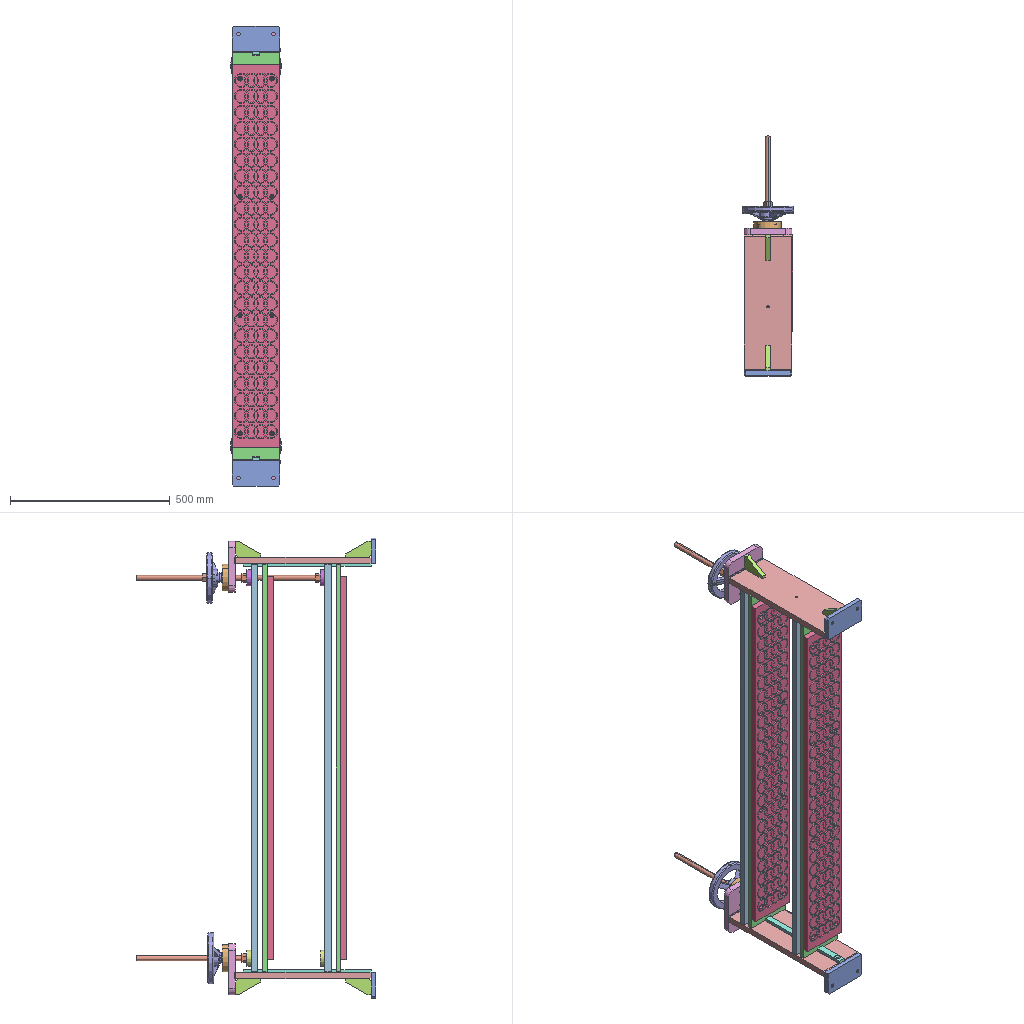Assembly | SolidWorks | 18 different items | 44 placed | box 160 x 749 x 1440 mm
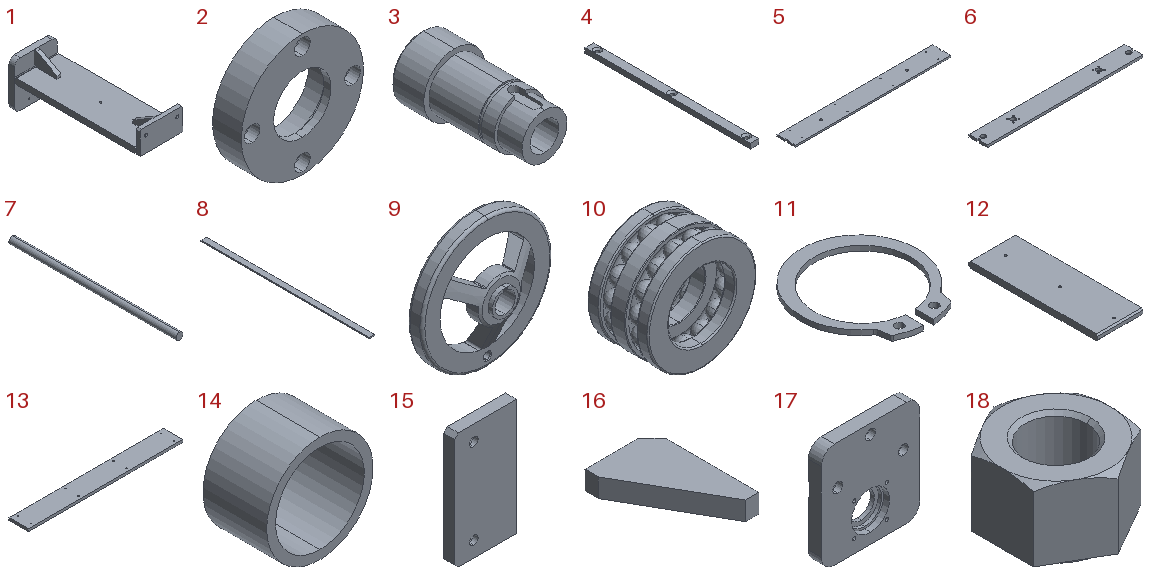Parts list (item | name | quantity | parent item | size | volume | features):
1 | (subassembly) | x2 | - | 150 x 460 x 170 mm | 1894202 mm3 | -
2 | - | x2 | - | 85 x 22 x 85 mm | 70234 mm3 | features ICE 4, Extrusion 1, HoleWzd 1
3 | - | x2 | - | 30 x 60 x 30 mm | 20081 mm3 | features ICE 3, Chamfer 1, HoleWzd 1, RevCut 1, Revolution 1
4 | - | x2 | in 1 | 20 x 400 x 12 mm | 92676 mm3 | features Extrusion 1, HoleWzd 1
5 | - | x2 | - | 1272 x 150 x 14 mm | 2656478 mm3 | features 3DProfileFeature 1, Extrusion 1, HoleWzd 1, ICE 1
6 | - | x2 | - | 1276 x 150 x 34 mm | 3757893 mm3 | features ICE 3, Cut 1, Extrusion 1
7 | - | x3 | - | 16 x 380 x 16 mm | 76404 mm3 | features Extrusion 1
8 | - | x2 | - | 10 x 300 x 2 mm | 6000 mm3 | features Extrusion 1
9 | - | x2 | - | 160 x 40 x 160 mm | 222311 mm3 | features ICE 4, MBimport 1
10 | - | x2 | - | 52 x 29 x 52 mm | 31888 mm3 | features Revolution 2, CirPattern 1
11 | - | x2 | - | 28.2 x 30.881 x 1.2 mm | 272.247 mm3 | features Extrusion 1
12 | - | x2 | in 1 | 150 x 426 x 20 mm | 1243356 mm3 | features Chamfer 2, HoleWzd 2, Extrusion 1, ICE 1
13 | - | x2 | - | 1200 x 150 x 20 mm | 3476597 mm3 | features LPattern 2, Extrusion 1, HoleWzd 1, ICE 1
14 | - | x2 | - | 30 x 18 x 30 mm | 3888 mm3 | features Extrusion 1
15 | - | x2 | in 1 | 80 x 14 x 150 mm | 162438 mm3 | features Chamfer 1, Extrusion 1, HoleWzd 1
16 | - | x4 | in 1 | 50 x 80 x 14 mm | 35700 mm3 | features Chamfer 1, Extrusion 1
17 | - | x2 | in 1 | 150 x 20 x 160 mm | 417009 mm3 | features ICE 4, HoleWzd 2, Extrusion 1, Fillet 1
18 | - | x7 | - | 24 x 27.713 x 16.4 mm | 5589 mm3 | features Cut 2, Chamfer 1, Extrusion 1
Mates (type | each side: item.copy, entity, surface, feature):
In the top assembly
Coincident | 12.1 face plane Boss-Extrude1 | 12.2 face plane Boss-Extrude1
Coincident | 15.1 face plane Boss-Extrude1 | 15.2 face plane Boss-Extrude1
Coincident | 17.1 face plane Boss-Extrude1 | 2.1 face plane Boss-Extrude1
Concentric | 17.1 face cylinder M6 Tapped Hole1 | 2.1 face cylinder M6 Clearance Hole1
Coincident | 17.2 face plane Boss-Extrude1 | 2.2 face plane Boss-Extrude1
Concentric | 17.2 face cylinder M6 Tapped Hole1 | 2.2 face cylinder M6 Clearance Hole1
DistanceDim | 6.1 face plane Boss-Extrude1 | 12.2 face plane Boss-Extrude1
DistanceDim | 6.1 face plane Boss-Extrude1 | 12.1 face plane Boss-Extrude1
Coincident | 12.2 face plane Boss-Extrude1 | 6.1 face plane Boss-Extrude1
DistanceDim | 6.1 face plane Boss-Extrude1 | 5.1 face plane Boss-Extrude1
Coincident | 6.1 face plane Boss-Extrude1 | 5.1 face plane Boss-Extrude1
Coincident | 5.1 face plane Boss-Extrude1 | 13.1 face plane Boss-Extrude1
Concentric | 5.1 face cylinder M8 Tapped Hole1 | 13.1 face cylinder Hole size (by socket head cap screw type)1 | 2 times
LimitDistanceDim | 13.1 face plane Boss-Extrude1 | 15.1 face plane Boss-Extrude1
Concentric | 6.1 face cylinder Cut-Extrude3 | 7.1 face cylinder Boss-Extrude1
DistanceDim | 7.1 face plane Boss-Extrude1 | 6.1 face plane Boss-Extrude1
Concentric | 6.1 face cylinder Cut-Extrude3 | 7.2 face cylinder Boss-Extrude1
Coincident | 7.1 face plane Boss-Extrude1 | 7.2 face plane Boss-Extrude1
Coincident | 17.1 face plane Cut-Extrude1 | 10.1 face plane Revolve1
Concentric | 17.1 face cylinder Cut-Extrude1 | 10.1 face cylinder Revolve1
Concentric | 17.2 face cylinder Cut-Extrude2 | 2.2 face cylinder Boss-Extrude3
Coincident | 3.1 face plane Revolve1 | 10.1 face plane Revolve1
Concentric | 3.1 face cylinder Revolve1 | 10.1 face cylinder Revolve1
Coincident | 10.1 face plane Revolve1 | 14.1 face plane Boss-Extrude1
Concentric | 3.1 face cylinder Revolve1 | 14.1 face cylinder Boss-Extrude1
Concentric | 7.2 face cylinder Boss-Extrude1 | 3.2 face cylinder Revolve1
Concentric | 7.1 face cylinder Boss-Extrude1 | 18.1 face cylinder Extrude1
Coincident | 6.1 face plane Boss-Extrude2 | 18.1 face plane Extrude1
Concentric | 7.2 face cylinder Boss-Extrude1 | 18.2 face cylinder Extrude1
Coincident | 6.1 face plane Boss-Extrude2 | 18.2 face plane Extrude1
Coincident | 6.1 face plane Boss-Extrude2 | 18.3 face plane Extrude1
Concentric | 7.1 face cylinder Boss-Extrude1 | 18.3 face cylinder Extrude1
Concentric | 7.2 face cylinder Boss-Extrude1 | 18.4 face cylinder Extrude1
Coincident | 6.1 face plane Boss-Extrude2 | 18.4 face plane Extrude1
Concentric | 7.2 face cylinder Boss-Extrude1 | 18.5 face cylinder Extrude1
Concentric | 7.1 face cylinder Boss-Extrude1 | 18.6 face cylinder Extrude1
Concentric | 3.2 face cylinder Revolve1 | 9.1 face cylinder Cut-Extrude3
DistanceDim | 9.1 face plane A cast iron flared handwheel [CTH306-160].step | 2.2 face plane Boss-Extrude1
Concentric | 3.1 face cylinder Revolve1 | 9.2 face cylinder Cut-Extrude3
DistanceDim | 9.1 face plane A cast iron flared handwheel [CTH306-160].step | 9.2 face plane A cast iron flared handwheel [CTH306-160].step
Coincident | 3.1 face plane Revolve1 | 3.2 face plane Revolve1
Coincident | 17.2 face plane Cut-Extrude1 | 10.2 face plane Revolve1
Concentric | 2.2 face cylinder Boss-Extrude1 | 10.2 face cylinder Revolve1
Coincident | 3.1 face plane Cut-Revolve1 | 11.1 face plane Base-Extrude
Concentric | 3.1 face cylinder Revolve1 | 11.1 face cylinder Base-Extrude
Coincident | 3.2 face plane Cut-Revolve1 | 11.2 face plane Base-Extrude
Concentric | 3.2 face cylinder Cut-Revolve1 | 11.2 face cylinder Base-Extrude
Coincident | 2.2 face plane Boss-Extrude1 | 14.2 face plane Boss-Extrude1
Concentric | 3.2 face cylinder Revolve1 | 14.2 face cylinder Boss-Extrude1
Coincident | 12.1 face plane Boss-Extrude1 | 8.1 face plane Boss-Extrude1 | 2 times
Coincident | 17.1 face plane Boss-Extrude1 | 8.1 face plane Boss-Extrude1
Coincident | 12.2 face plane Boss-Extrude1 | 8.2 face plane Boss-Extrude1 | 2 times
Coincident | 17.2 face plane Boss-Extrude1 | 8.2 face plane Boss-Extrude1
In subassembly 1
Coincident | 12.3 face plane Boss-Extrude1 | 15.3 face plane Boss-Extrude1 | 3 times
Coincident | 15.3 face plane Boss-Extrude1 | 16.1 face plane Boss-Extrude1
Width | 16.1 face plane Boss-Extrude1 | 16.1 face plane Boss-Extrude1 | 12.3 face plane Boss-Extrude1 | 12.3 face plane Boss-Extrude1
Coincident | 12.3 face plane Boss-Extrude1 | 16.1 face plane Boss-Extrude1
Coincident | 12.3 face plane Cut-Extrude1 | 4.1 face plane Boss-Extrude1 | 2 times
Coincident | 12.3 face plane Boss-Extrude1 | 17.3 face plane Boss-Extrude1 | 2 times
Coincident | 15.3 face plane Boss-Extrude1 | 4.1 face plane Boss-Extrude1
Coincident | 17.3 face plane Boss-Extrude1 | 16.2 face plane Boss-Extrude1 | 2 times
Coincident | 16.1 face plane Boss-Extrude1 | 16.2 face plane Boss-Extrude1 | 2 times